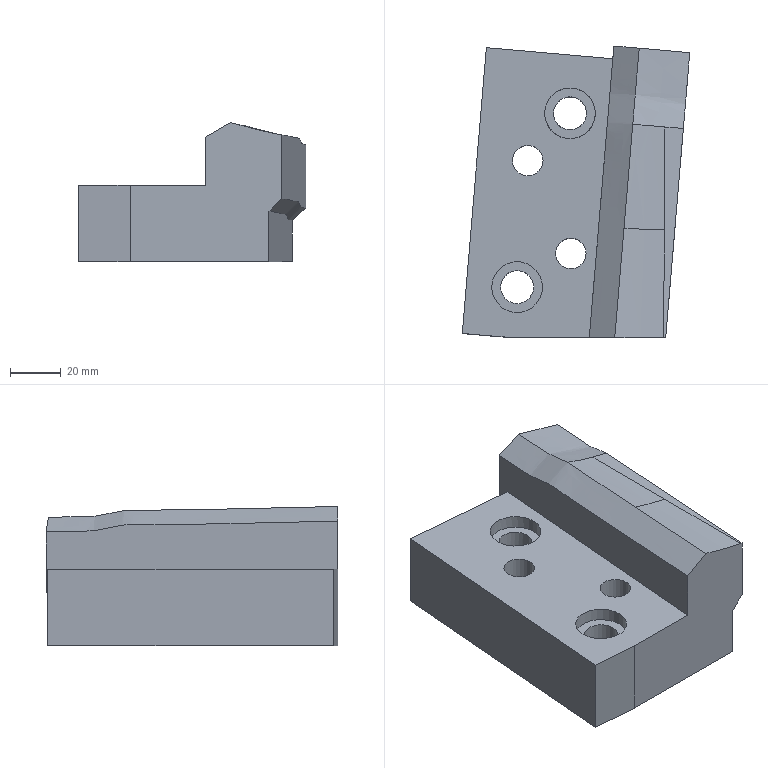Part | NX | features solid 2 | 1 solid | 27 faces | box 89.619 x 114.935 x 54.761 mm | volume 310420 mm3 | plane 15 | spline 6 | cylinder 6 | commonest cylinder face diameters 12 x2 13 x2 20 x2